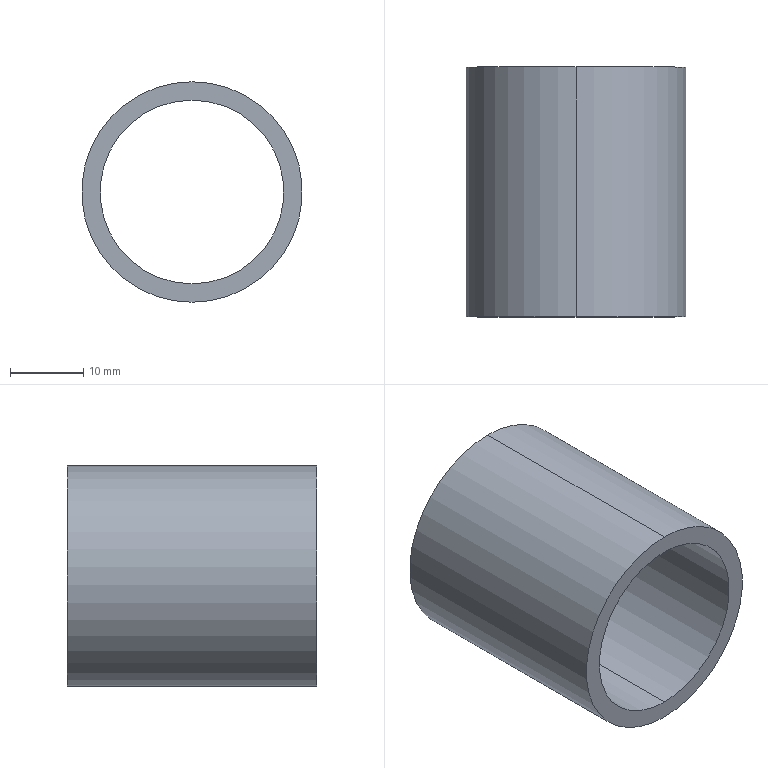Part | SolidWorks | features Extrusion 1 | 1 solid | 6 faces | box 30 x 34 x 30 mm | volume 7343 mm3 | cylinder 4 | plane 2 | commonest cylinder face diameters 25 x2 30 x2
STEP:
#1=CARTESIAN_POINT('',(0.,34.,-12.5));
#2=VERTEX_POINT('',#1);
#3=CARTESIAN_POINT('',(0.,34.,12.5));
#4=VERTEX_POINT('',#3);
#5=CARTESIAN_POINT('',(0.,34.,0.));
#6=DIRECTION('',(0.,1.,0.));
#7=DIRECTION('',(0.,0.,1.));
#8=AXIS2_PLACEMENT_3D('',#5,#6,#7);
#9=CIRCLE('',#8,12.5);
#10=EDGE_CURVE('',#2,#4,#9,.T.);
#11=ORIENTED_EDGE('',*,*,#10,.T.);
#12=CARTESIAN_POINT('',(0.,0.,12.5));
#13=VERTEX_POINT('',#12);
#14=CARTESIAN_POINT('',(0.,34.,12.5));
#15=DIRECTION('',(0.,-1.,0.));
#16=VECTOR('',#15,1000.);
#17=LINE('',#14,#16);
#18=EDGE_CURVE('',#4,#13,#17,.T.);
#19=ORIENTED_EDGE('',*,*,#18,.T.);
#20=CARTESIAN_POINT('',(0.,0.,-12.5));
#21=VERTEX_POINT('',#20);
#22=CARTESIAN_POINT('',(0.,0.,0.));
#23=DIRECTION('',(0.,1.,0.));
#24=DIRECTION('',(0.,0.,1.));
#25=AXIS2_PLACEMENT_3D('',#22,#23,#24);
#26=CIRCLE('',#25,12.5);
#27=EDGE_CURVE('',#21,#13,#26,.T.);
#28=ORIENTED_EDGE('',*,*,#27,.F.);
#29=CARTESIAN_POINT('',(0.,34.,-12.5));
#30=DIRECTION('',(0.,-1.,0.));
#31=VECTOR('',#30,1000.);
#32=LINE('',#29,#31);
#33=EDGE_CURVE('',#2,#21,#32,.T.);
#34=ORIENTED_EDGE('',*,*,#33,.F.);
#35=EDGE_LOOP('',(#11,#19,#28,#34));
#36=FACE_OUTER_BOUND('',#35,.T.);
#37=CARTESIAN_POINT('',(0.,34.,0.));
#38=DIRECTION('',(0.,-1.,0.));
#39=DIRECTION('',(0.,0.,-1.));
#40=AXIS2_PLACEMENT_3D('',#37,#38,#39);
#41=CYLINDRICAL_SURFACE('',#40,12.5);
#42=ADVANCED_FACE('',(#36),#41,.F.);
#43=CARTESIAN_POINT('',(0.,34.,15.));
#44=VERTEX_POINT('',#43);
#45=CARTESIAN_POINT('',(0.,34.,-15.));
#46=VERTEX_POINT('',#45);
#47=CARTESIAN_POINT('',(0.,34.,0.));
#48=DIRECTION('',(0.,1.,0.));
#49=DIRECTION('',(0.,0.,1.));
#50=AXIS2_PLACEMENT_3D('',#47,#48,#49);
#51=CIRCLE('',#50,15.);
#52=EDGE_CURVE('',#44,#46,#51,.T.);
#53=ORIENTED_EDGE('',*,*,#52,.F.);
#54=CARTESIAN_POINT('',(0.,0.,15.));
#55=VERTEX_POINT('',#54);
#56=CARTESIAN_POINT('',(0.,34.,15.));
#57=DIRECTION('',(0.,-1.,0.));
#58=VECTOR('',#57,1000.);
#59=LINE('',#56,#58);
#60=EDGE_CURVE('',#44,#55,#59,.T.);
#61=ORIENTED_EDGE('',*,*,#60,.T.);
#62=CARTESIAN_POINT('',(0.,0.,-15.));
#63=VERTEX_POINT('',#62);
#64=CARTESIAN_POINT('',(0.,0.,0.));
#65=DIRECTION('',(0.,1.,0.));
#66=DIRECTION('',(0.,0.,1.));
#67=AXIS2_PLACEMENT_3D('',#64,#65,#66);
#68=CIRCLE('',#67,15.);
#69=EDGE_CURVE('',#55,#63,#68,.T.);
#70=ORIENTED_EDGE('',*,*,#69,.T.);
#71=CARTESIAN_POINT('',(0.,34.,-15.));
#72=DIRECTION('',(0.,-1.,0.));
#73=VECTOR('',#72,1000.);
#74=LINE('',#71,#73);
#75=EDGE_CURVE('',#46,#63,#74,.T.);
#76=ORIENTED_EDGE('',*,*,#75,.F.);
#77=EDGE_LOOP('',(#53,#61,#70,#76));
#78=FACE_OUTER_BOUND('',#77,.T.);
#79=CARTESIAN_POINT('',(0.,34.,0.));
#80=DIRECTION('',(0.,-1.,0.));
#81=DIRECTION('',(0.,0.,-1.));
#82=AXIS2_PLACEMENT_3D('',#79,#80,#81);
#83=CYLINDRICAL_SURFACE('',#82,15.);
#84=ADVANCED_FACE('',(#78),#83,.T.);
#85=CARTESIAN_POINT('',(0.,34.,0.));
#86=DIRECTION('',(0.,1.,0.));
#87=DIRECTION('',(0.,0.,1.));
#88=AXIS2_PLACEMENT_3D('',#85,#86,#87);
#89=CIRCLE('',#88,15.);
#90=EDGE_CURVE('',#46,#44,#89,.T.);
#91=ORIENTED_EDGE('',*,*,#90,.T.);
#92=ORIENTED_EDGE('',*,*,#52,.T.);
#93=EDGE_LOOP('',(#91,#92));
#94=FACE_OUTER_BOUND('',#93,.T.);
#95=ORIENTED_EDGE('',*,*,#10,.F.);
#96=CARTESIAN_POINT('',(0.,34.,0.));
#97=DIRECTION('',(0.,1.,0.));
#98=DIRECTION('',(0.,0.,1.));
#99=AXIS2_PLACEMENT_3D('',#96,#97,#98);
#100=CIRCLE('',#99,12.5);
#101=EDGE_CURVE('',#4,#2,#100,.T.);
#102=ORIENTED_EDGE('',*,*,#101,.F.);
#103=EDGE_LOOP('',(#95,#102));
#104=FACE_BOUND('',#103,.T.);
#105=CARTESIAN_POINT('',(0.,34.,0.));
#106=DIRECTION('',(0.,1.,0.));
#107=DIRECTION('',(0.,0.,1.));
#108=AXIS2_PLACEMENT_3D('',#105,#106,#107);
#109=PLANE('',#108);
#110=ADVANCED_FACE('',(#94,#104),#109,.T.);
#111=CARTESIAN_POINT('',(0.,0.,0.));
#112=DIRECTION('',(0.,1.,0.));
#113=DIRECTION('',(0.,0.,1.));
#114=AXIS2_PLACEMENT_3D('',#111,#112,#113);
#115=CIRCLE('',#114,15.);
#116=EDGE_CURVE('',#63,#55,#115,.T.);
#117=ORIENTED_EDGE('',*,*,#116,.F.);
#118=ORIENTED_EDGE('',*,*,#69,.F.);
#119=EDGE_LOOP('',(#117,#118));
#120=FACE_OUTER_BOUND('',#119,.T.);
#121=ORIENTED_EDGE('',*,*,#27,.T.);
#122=CARTESIAN_POINT('',(0.,0.,0.));
#123=DIRECTION('',(0.,1.,0.));
#124=DIRECTION('',(0.,0.,1.));
#125=AXIS2_PLACEMENT_3D('',#122,#123,#124);
#126=CIRCLE('',#125,12.5);
#127=EDGE_CURVE('',#13,#21,#126,.T.);
#128=ORIENTED_EDGE('',*,*,#127,.T.);
#129=EDGE_LOOP('',(#121,#128));
#130=FACE_BOUND('',#129,.T.);
#131=CARTESIAN_POINT('',(0.,0.,0.));
#132=DIRECTION('',(0.,1.,0.));
#133=DIRECTION('',(0.,0.,1.));
#134=AXIS2_PLACEMENT_3D('',#131,#132,#133);
#135=PLANE('',#134);
#136=ADVANCED_FACE('',(#120,#130),#135,.F.);
#137=ORIENTED_EDGE('',*,*,#60,.F.);
#138=ORIENTED_EDGE('',*,*,#90,.F.);
#139=ORIENTED_EDGE('',*,*,#75,.T.);
#140=ORIENTED_EDGE('',*,*,#116,.T.);
#141=EDGE_LOOP('',(#137,#138,#139,#140));
#142=FACE_OUTER_BOUND('',#141,.T.);
#143=CARTESIAN_POINT('',(0.,34.,0.));
#144=DIRECTION('',(0.,-1.,0.));
#145=DIRECTION('',(0.,0.,-1.));
#146=AXIS2_PLACEMENT_3D('',#143,#144,#145);
#147=CYLINDRICAL_SURFACE('',#146,15.);
#148=ADVANCED_FACE('',(#142),#147,.T.);
#149=ORIENTED_EDGE('',*,*,#18,.F.);
#150=ORIENTED_EDGE('',*,*,#101,.T.);
#151=ORIENTED_EDGE('',*,*,#33,.T.);
#152=ORIENTED_EDGE('',*,*,#127,.F.);
#153=EDGE_LOOP('',(#149,#150,#151,#152));
#154=FACE_OUTER_BOUND('',#153,.T.);
#155=CARTESIAN_POINT('',(0.,34.,0.));
#156=DIRECTION('',(0.,-1.,0.));
#157=DIRECTION('',(0.,0.,-1.));
#158=AXIS2_PLACEMENT_3D('',#155,#156,#157);
#159=CYLINDRICAL_SURFACE('',#158,12.5);
#160=ADVANCED_FACE('',(#154),#159,.F.);
#161=CLOSED_SHELL('',(#42,#84,#110,#136,#148,#160));
#162=MANIFOLD_SOLID_BREP('',#161);
#163=CARTESIAN_POINT('',(0.,0.,0.));
#164=DIRECTION('',(0.,0.,1.));
#165=DIRECTION('',(1.,0.,0.));
#166=AXIS2_PLACEMENT_3D('',#163,#164,#165);
#167=(LENGTH_UNIT()NAMED_UNIT(*)SI_UNIT(.MILLI.,.METRE.));
#168=UNCERTAINTY_MEASURE_WITH_UNIT(LENGTH_MEASURE(0.00001),#167,'','');
#169=(NAMED_UNIT(*)PLANE_ANGLE_UNIT()SI_UNIT($,.RADIAN.));
#170=(NAMED_UNIT(*)SI_UNIT($,.STERADIAN.)SOLID_ANGLE_UNIT());
#171=(GEOMETRIC_REPRESENTATION_CONTEXT(3)GLOBAL_UNCERTAINTY_ASSIGNED_CONTEXT((#168))GLOBAL_UNIT_ASSIGNED_CONTEXT((#167,#169,#170))REPRESENTATION_CONTEXT('',''));
#172=ADVANCED_BREP_SHAPE_REPRESENTATION('',(#162,#166),#171);